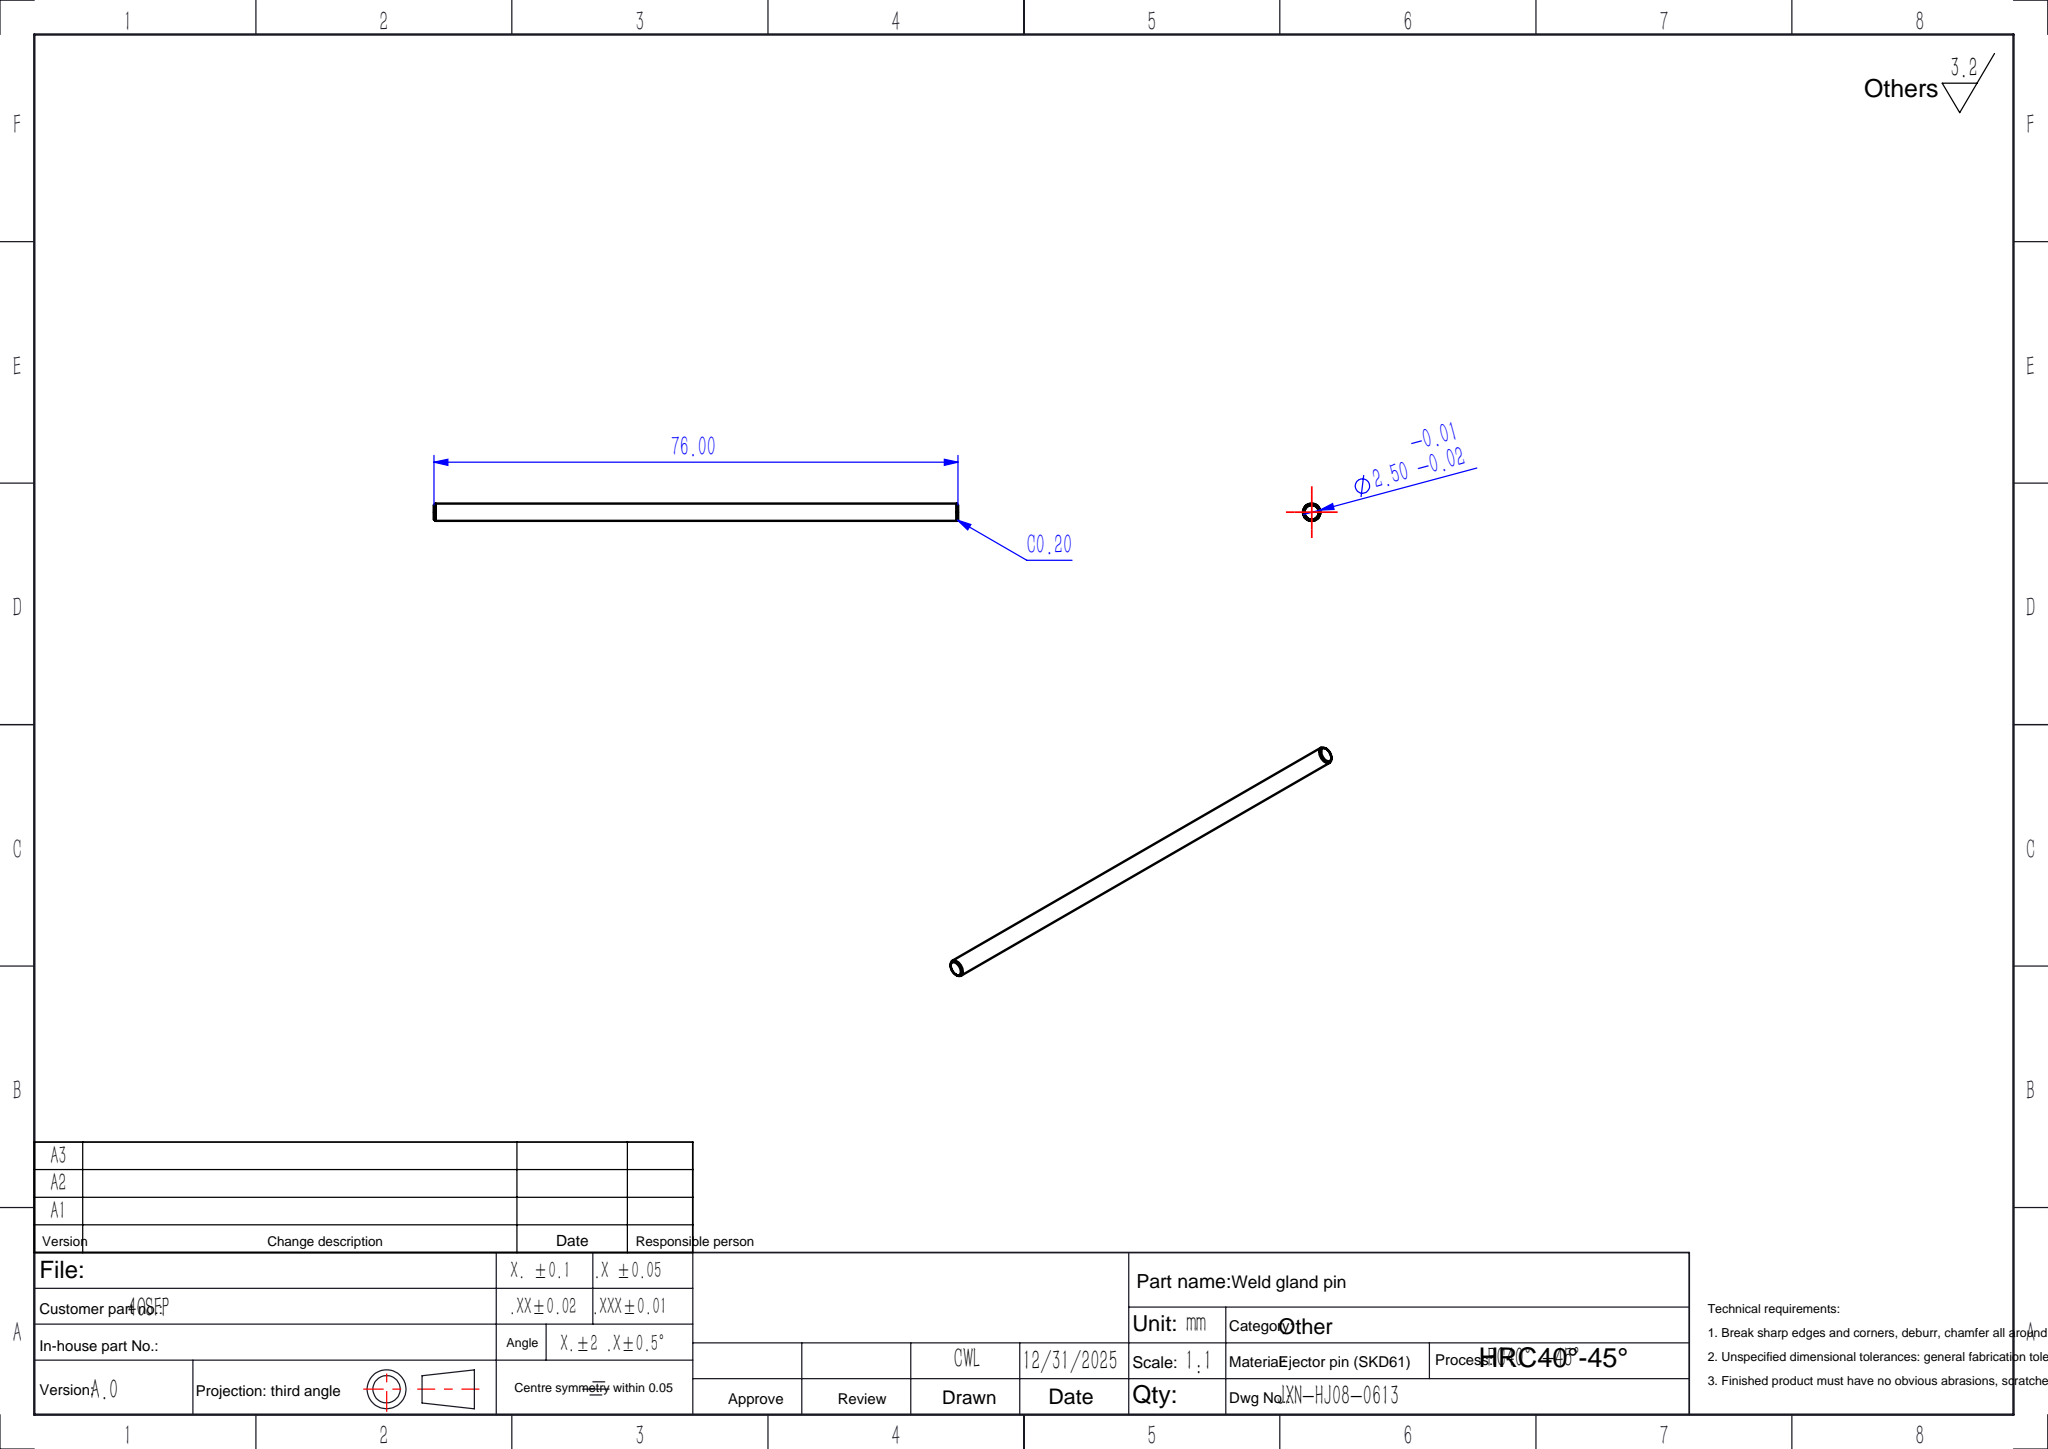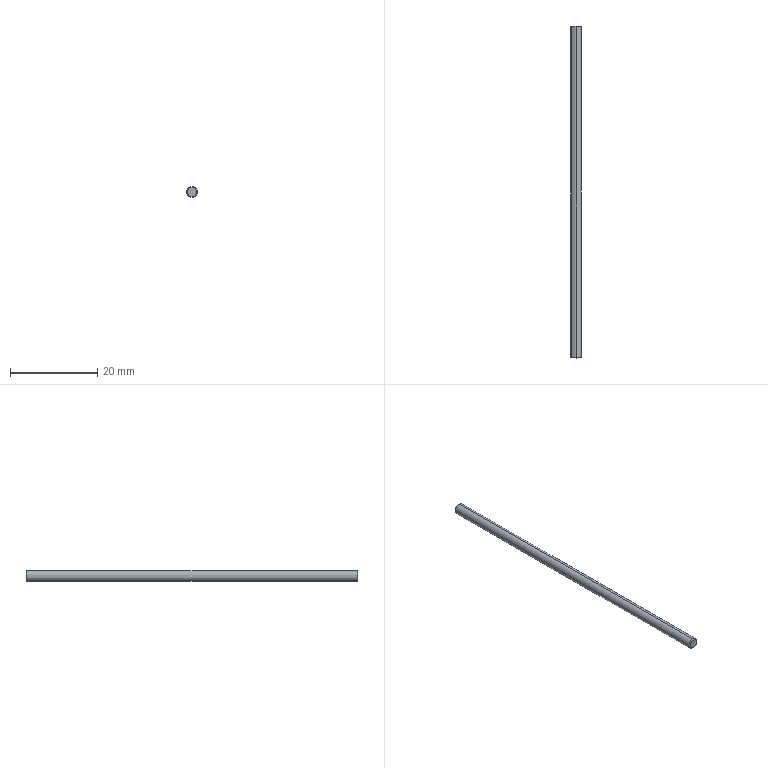Part | SolidWorks | features Chamfer 1, Extrusion 1 | 1 solid | 8 faces | box 2.5 x 76 x 2.5 mm | volume 372.767 mm3 | cone 4 | cylinder 2 | plane 2 | commonest cylinder face diameters 2.5 x2
STEP:
#1=CARTESIAN_POINT('',(0.,0.,-1.05));
#2=VERTEX_POINT('',#1);
#3=CARTESIAN_POINT('',(0.,0.,1.05));
#4=VERTEX_POINT('',#3);
#5=CARTESIAN_POINT('',(0.,0.,0.));
#6=DIRECTION('',(0.,-1.,0.));
#7=DIRECTION('',(0.,0.,1.));
#8=AXIS2_PLACEMENT_3D('',#5,#6,#7);
#9=CIRCLE('',#8,1.05);
#10=EDGE_CURVE('',#2,#4,#9,.T.);
#11=ORIENTED_EDGE('',*,*,#10,.F.);
#12=CARTESIAN_POINT('',(0.,0.2,-1.25));
#13=VERTEX_POINT('',#12);
#14=CARTESIAN_POINT('',(0.,0.2,-1.25));
#15=DIRECTION('',(0.,0.7071,-0.7071));
#16=VECTOR('',#15,1000.);
#17=LINE('',#14,#16);
#18=EDGE_CURVE('',#2,#13,#17,.T.);
#19=ORIENTED_EDGE('',*,*,#18,.T.);
#20=CARTESIAN_POINT('',(0.,0.2,1.25));
#21=VERTEX_POINT('',#20);
#22=CARTESIAN_POINT('',(0.,0.2,0.));
#23=DIRECTION('',(0.,1.,0.));
#24=DIRECTION('',(0.,0.,1.));
#25=AXIS2_PLACEMENT_3D('',#22,#23,#24);
#26=CIRCLE('',#25,1.25);
#27=EDGE_CURVE('',#21,#13,#26,.T.);
#28=ORIENTED_EDGE('',*,*,#27,.F.);
#29=CARTESIAN_POINT('',(0.,0.2,1.25));
#30=DIRECTION('',(0.,0.7071,0.7071));
#31=VECTOR('',#30,1000.);
#32=LINE('',#29,#31);
#33=EDGE_CURVE('',#4,#21,#32,.T.);
#34=ORIENTED_EDGE('',*,*,#33,.F.);
#35=EDGE_LOOP('',(#11,#19,#28,#34));
#36=FACE_OUTER_BOUND('',#35,.T.);
#37=CARTESIAN_POINT('',(0.,0.2,0.));
#38=DIRECTION('',(0.,1.,0.));
#39=DIRECTION('',(0.,0.,1.));
#40=AXIS2_PLACEMENT_3D('',#37,#38,#39);
#41=CONICAL_SURFACE('',#40,1.25,0.7854);
#42=ADVANCED_FACE('',(#36),#41,.T.);
#43=CARTESIAN_POINT('',(0.,76.,1.05));
#44=VERTEX_POINT('',#43);
#45=CARTESIAN_POINT('',(0.,76.,-1.05));
#46=VERTEX_POINT('',#45);
#47=CARTESIAN_POINT('',(0.,76.,0.));
#48=DIRECTION('',(0.,1.,0.));
#49=DIRECTION('',(0.,0.,1.));
#50=AXIS2_PLACEMENT_3D('',#47,#48,#49);
#51=CIRCLE('',#50,1.05);
#52=EDGE_CURVE('',#44,#46,#51,.T.);
#53=ORIENTED_EDGE('',*,*,#52,.F.);
#54=CARTESIAN_POINT('',(0.,75.8,1.25));
#55=VERTEX_POINT('',#54);
#56=CARTESIAN_POINT('',(0.,76.,1.05));
#57=DIRECTION('',(0.,-0.7071,0.7071));
#58=VECTOR('',#57,1000.);
#59=LINE('',#56,#58);
#60=EDGE_CURVE('',#44,#55,#59,.T.);
#61=ORIENTED_EDGE('',*,*,#60,.T.);
#62=CARTESIAN_POINT('',(0.,75.8,-1.25));
#63=VERTEX_POINT('',#62);
#64=CARTESIAN_POINT('',(0.,75.8,0.));
#65=DIRECTION('',(0.,-1.,0.));
#66=DIRECTION('',(0.,0.,1.));
#67=AXIS2_PLACEMENT_3D('',#64,#65,#66);
#68=CIRCLE('',#67,1.25);
#69=EDGE_CURVE('',#63,#55,#68,.T.);
#70=ORIENTED_EDGE('',*,*,#69,.F.);
#71=CARTESIAN_POINT('',(0.,76.,-1.05));
#72=DIRECTION('',(0.,-0.7071,-0.7071));
#73=VECTOR('',#72,1000.);
#74=LINE('',#71,#73);
#75=EDGE_CURVE('',#46,#63,#74,.T.);
#76=ORIENTED_EDGE('',*,*,#75,.F.);
#77=EDGE_LOOP('',(#53,#61,#70,#76));
#78=FACE_OUTER_BOUND('',#77,.T.);
#79=CARTESIAN_POINT('',(0.,76.,0.));
#80=DIRECTION('',(0.,-1.,0.));
#81=DIRECTION('',(0.,0.,-1.));
#82=AXIS2_PLACEMENT_3D('',#79,#80,#81);
#83=CONICAL_SURFACE('',#82,1.05,0.7854);
#84=ADVANCED_FACE('',(#78),#83,.T.);
#85=ORIENTED_EDGE('',*,*,#69,.T.);
#86=CARTESIAN_POINT('',(0.,76.,1.25));
#87=DIRECTION('',(0.,-1.,0.));
#88=VECTOR('',#87,1000.);
#89=LINE('',#86,#88);
#90=EDGE_CURVE('',#55,#21,#89,.T.);
#91=ORIENTED_EDGE('',*,*,#90,.T.);
#92=ORIENTED_EDGE('',*,*,#27,.T.);
#93=CARTESIAN_POINT('',(0.,76.,-1.25));
#94=DIRECTION('',(0.,-1.,0.));
#95=VECTOR('',#94,1000.);
#96=LINE('',#93,#95);
#97=EDGE_CURVE('',#63,#13,#96,.T.);
#98=ORIENTED_EDGE('',*,*,#97,.F.);
#99=EDGE_LOOP('',(#85,#91,#92,#98));
#100=FACE_OUTER_BOUND('',#99,.T.);
#101=CARTESIAN_POINT('',(0.,76.,0.));
#102=DIRECTION('',(0.,-1.,0.));
#103=DIRECTION('',(0.,0.,-1.));
#104=AXIS2_PLACEMENT_3D('',#101,#102,#103);
#105=CYLINDRICAL_SURFACE('',#104,1.25);
#106=ADVANCED_FACE('',(#100),#105,.T.);
#107=ORIENTED_EDGE('',*,*,#90,.F.);
#108=CARTESIAN_POINT('',(0.,75.8,0.));
#109=DIRECTION('',(0.,-1.,0.));
#110=DIRECTION('',(0.,0.,1.));
#111=AXIS2_PLACEMENT_3D('',#108,#109,#110);
#112=CIRCLE('',#111,1.25);
#113=EDGE_CURVE('',#55,#63,#112,.T.);
#114=ORIENTED_EDGE('',*,*,#113,.T.);
#115=ORIENTED_EDGE('',*,*,#97,.T.);
#116=CARTESIAN_POINT('',(0.,0.2,0.));
#117=DIRECTION('',(0.,1.,0.));
#118=DIRECTION('',(0.,0.,1.));
#119=AXIS2_PLACEMENT_3D('',#116,#117,#118);
#120=CIRCLE('',#119,1.25);
#121=EDGE_CURVE('',#13,#21,#120,.T.);
#122=ORIENTED_EDGE('',*,*,#121,.T.);
#123=EDGE_LOOP('',(#107,#114,#115,#122));
#124=FACE_OUTER_BOUND('',#123,.T.);
#125=CARTESIAN_POINT('',(0.,76.,0.));
#126=DIRECTION('',(0.,-1.,0.));
#127=DIRECTION('',(0.,0.,-1.));
#128=AXIS2_PLACEMENT_3D('',#125,#126,#127);
#129=CYLINDRICAL_SURFACE('',#128,1.25);
#130=ADVANCED_FACE('',(#124),#129,.T.);
#131=CARTESIAN_POINT('',(0.,76.,0.));
#132=DIRECTION('',(0.,1.,0.));
#133=DIRECTION('',(0.,0.,1.));
#134=AXIS2_PLACEMENT_3D('',#131,#132,#133);
#135=CIRCLE('',#134,1.05);
#136=EDGE_CURVE('',#46,#44,#135,.T.);
#137=ORIENTED_EDGE('',*,*,#136,.T.);
#138=ORIENTED_EDGE('',*,*,#52,.T.);
#139=EDGE_LOOP('',(#137,#138));
#140=FACE_OUTER_BOUND('',#139,.T.);
#141=CARTESIAN_POINT('',(0.,76.,0.));
#142=DIRECTION('',(0.,1.,0.));
#143=DIRECTION('',(0.,0.,1.));
#144=AXIS2_PLACEMENT_3D('',#141,#142,#143);
#145=PLANE('',#144);
#146=ADVANCED_FACE('',(#140),#145,.T.);
#147=CARTESIAN_POINT('',(0.,0.,0.));
#148=DIRECTION('',(0.,-1.,0.));
#149=DIRECTION('',(0.,0.,1.));
#150=AXIS2_PLACEMENT_3D('',#147,#148,#149);
#151=CIRCLE('',#150,1.05);
#152=EDGE_CURVE('',#4,#2,#151,.T.);
#153=ORIENTED_EDGE('',*,*,#152,.T.);
#154=ORIENTED_EDGE('',*,*,#10,.T.);
#155=EDGE_LOOP('',(#153,#154));
#156=FACE_OUTER_BOUND('',#155,.T.);
#157=CARTESIAN_POINT('',(0.,0.,0.));
#158=DIRECTION('',(0.,1.,0.));
#159=DIRECTION('',(0.,0.,1.));
#160=AXIS2_PLACEMENT_3D('',#157,#158,#159);
#161=PLANE('',#160);
#162=ADVANCED_FACE('',(#156),#161,.F.);
#163=ORIENTED_EDGE('',*,*,#60,.F.);
#164=ORIENTED_EDGE('',*,*,#136,.F.);
#165=ORIENTED_EDGE('',*,*,#75,.T.);
#166=ORIENTED_EDGE('',*,*,#113,.F.);
#167=EDGE_LOOP('',(#163,#164,#165,#166));
#168=FACE_OUTER_BOUND('',#167,.T.);
#169=CARTESIAN_POINT('',(0.,76.,0.));
#170=DIRECTION('',(0.,-1.,0.));
#171=DIRECTION('',(0.,0.,-1.));
#172=AXIS2_PLACEMENT_3D('',#169,#170,#171);
#173=CONICAL_SURFACE('',#172,1.05,0.7854);
#174=ADVANCED_FACE('',(#168),#173,.T.);
#175=ORIENTED_EDGE('',*,*,#18,.F.);
#176=ORIENTED_EDGE('',*,*,#152,.F.);
#177=ORIENTED_EDGE('',*,*,#33,.T.);
#178=ORIENTED_EDGE('',*,*,#121,.F.);
#179=EDGE_LOOP('',(#175,#176,#177,#178));
#180=FACE_OUTER_BOUND('',#179,.T.);
#181=CARTESIAN_POINT('',(0.,0.2,0.));
#182=DIRECTION('',(0.,1.,0.));
#183=DIRECTION('',(0.,0.,1.));
#184=AXIS2_PLACEMENT_3D('',#181,#182,#183);
#185=CONICAL_SURFACE('',#184,1.25,0.7854);
#186=ADVANCED_FACE('',(#180),#185,.T.);
#187=CLOSED_SHELL('',(#42,#84,#106,#130,#146,#162,#174,#186));
#188=MANIFOLD_SOLID_BREP('',#187);
#189=CARTESIAN_POINT('',(0.,0.,0.));
#190=DIRECTION('',(0.,0.,1.));
#191=DIRECTION('',(1.,0.,0.));
#192=AXIS2_PLACEMENT_3D('',#189,#190,#191);
#193=(LENGTH_UNIT()NAMED_UNIT(*)SI_UNIT(.MILLI.,.METRE.));
#194=UNCERTAINTY_MEASURE_WITH_UNIT(LENGTH_MEASURE(0.00001),#193,'','');
#195=(NAMED_UNIT(*)PLANE_ANGLE_UNIT()SI_UNIT($,.RADIAN.));
#196=(NAMED_UNIT(*)SI_UNIT($,.STERADIAN.)SOLID_ANGLE_UNIT());
#197=(GEOMETRIC_REPRESENTATION_CONTEXT(3)GLOBAL_UNCERTAINTY_ASSIGNED_CONTEXT((#194))GLOBAL_UNIT_ASSIGNED_CONTEXT((#193,#195,#196))REPRESENTATION_CONTEXT('',''));
#198=ADVANCED_BREP_SHAPE_REPRESENTATION('',(#188,#192),#197);